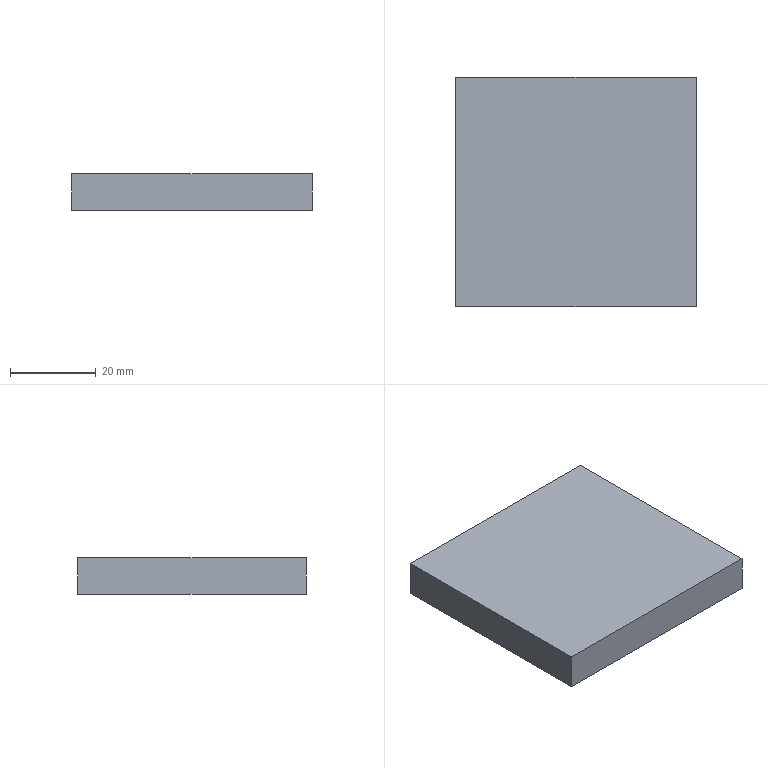NC program | NX | posted with a generic post | part box 56 x 53.3 x 8.5 mm
Lines 35 to 843 of 5023:
(刀补11_COPY_1_COPY , TOOL : D6)
N68 T12 M6
N70 G54
N72 G17 G0 G90 X5.148 Y-24.207 S9500 M3
N74 G43 Z30. H12
N76 Z1.5
N78 G94 G1 X3.722 Y-24.479 Z1.424 F1000.
N80 X1.866 Y-24.69 Z1.326
N82 X0. Y-24.76 Z1.228
N84 X-1.866 Y-24.69 Z1.13
N86 X-3.722 Y-24.479 Z1.032
N88 X-5.556 Y-24.129 Z0.935
N90 X-7.359 Y-23.641 Z0.837
N92 X-9.12 Y-23.019 Z0.739
N94 X-10.828 Y-22.267 Z0.641
N96 X-12.476 Y-21.387 Z0.543
N98 X-13.358 Y-20.839 Z0.489
N100 X-14.002 Y-20.306 Z0.445
N102 X-14.559 Y-19.684 Z0.401
N104 X-15.018 Y-18.987 Z0.357
N106 X-15.369 Y-18.228 Z0.314
N108 X-15.603 Y-17.426 Z0.27
N110 X-15.715 Y-16.598 Z0.226
N112 Y-15.974 Z0.193
N114 X-15.686 Y-15.686 Z0.178
N116 X-16.019 Y-15.72 Z0.161
N118 X-16.95 Y-15.683 Z0.112
N120 X-17.862 Y-15.492 Z0.063
N122 X-18.73 Y-15.153 Z0.014
N124 X-19.529 Y-14.675 Z-0.035
N126 X-20.239 Y-14.071 Z-0.084
N128 X-20.839 Y-13.358 Z-0.132
N130 X-21.015 Y-13.073 Z-0.15
N132 G2 X-22.44 Y-10.442 R24.75 F2000.
N134 X-24.805 Y-8.12 R3.6
N136 X-24.805 Y8.12 R26.1
N138 X-22.44 Y10.442 R3.6
N140 X-21.015 Y13.073 R24.75
N142 X-15.686 Y15.686 R5.6
N144 X-13.073 Y21.015 R5.6
N146 X13.073 Y21.015 R24.75
N148 X15.686 Y15.686 R5.6
N150 X21.015 Y13.073 R5.6
N152 X22.44 Y10.442 R24.75
N154 X24.805 Y8.12 R3.6
N156 X24.805 Y-8.12 R26.1
N158 X22.44 Y-10.442 R3.6
N160 X21.015 Y-13.073 R24.75
N162 X15.686 Y-15.686 R5.6
N164 X13.073 Y-21.015 R5.6
N166 X-13.073 Y-21.015 R24.75
N168 X-15.686 Y-15.686 R5.6
N170 X-21.015 Y-13.073 R5.6
N172 G1 X-21.106 Y-12.927 Z-0.153
N174 X-21.195 Y-12.78 Z-0.156
N176 X-21.283 Y-12.633 Z-0.159
N178 X-21.37 Y-12.485 Z-0.162
N180 X-21.457 Y-12.336 Z-0.165
N182 X-21.542 Y-12.187 Z-0.168
N184 X-21.626 Y-12.037 Z-0.171
N186 X-21.709 Y-11.886 Z-0.174
N188 X-21.791 Y-11.735 Z-0.177
N190 X-21.872 Y-11.584 Z-0.18
N192 X-21.952 Y-11.431 Z-0.183
N194 X-22.031 Y-11.279 Z-0.186
N196 X-22.109 Y-11.126 Z-0.189
N198 X-22.185 Y-10.972 Z-0.192
N200 X-22.261 Y-10.817 Z-0.195
N202 X-22.335 Y-10.663 Z-0.198
N204 X-22.437 Y-10.447 Z-0.202
N206 X-22.534 Y-10.411 Z-0.204
N208 X-22.696 Y-10.352 Z-0.207
N210 X-22.854 Y-10.286 Z-0.21
N212 X-23.009 Y-10.212 Z-0.213
N214 X-23.161 Y-10.131 Z-0.216
N216 X-23.308 Y-10.042 Z-0.219
N218 X-23.451 Y-9.947 Z-0.222
N220 X-23.589 Y-9.845 Z-0.225
N222 X-23.723 Y-9.736 Z-0.228
N224 X-23.851 Y-9.622 Z-0.231
N226 X-23.973 Y-9.501 Z-0.234
N228 X-24.089 Y-9.374 Z-0.237
N230 X-24.2 Y-9.243 Z-0.24
N232 X-24.303 Y-9.106 Z-0.243
N234 X-24.401 Y-8.964 Z-0.246
N236 X-24.491 Y-8.818 Z-0.249
N238 X-24.574 Y-8.667 Z-0.252
N240 X-24.65 Y-8.513 Z-0.255
N242 X-24.718 Y-8.356 Z-0.258
N244 X-24.779 Y-8.195 Z-0.261
N246 X-24.833 Y-8.032 Z-0.264
N248 X-24.886 Y-7.868 Z-0.267
N250 X-24.937 Y-7.704 Z-0.27
N252 X-24.987 Y-7.54 Z-0.273
N254 X-25.036 Y-7.375 Z-0.276
N256 X-25.084 Y-7.21 Z-0.279
N258 X-25.131 Y-7.044 Z-0.282
N260 X-25.177 Y-6.879 Z-0.285
N262 X-25.222 Y-6.713 Z-0.288
N264 X-25.266 Y-6.547 Z-0.291
N266 X-25.308 Y-6.38 Z-0.294
N268 X-25.35 Y-6.213 Z-0.297
N270 X-25.39 Y-6.046 Z-0.3
N272 G2 X-24.805 Y8.12 R26.1
N274 X-22.44 Y10.442 R3.6
N276 X-21.015 Y13.073 R24.75
N278 X-15.686 Y15.686 R5.6
N280 X-13.073 Y21.015 R5.6
N282 X13.073 Y21.015 R24.75
N284 X15.686 Y15.686 R5.6
N286 X21.015 Y13.073 R5.6
N288 X22.44 Y10.442 R24.75
N290 X24.805 Y8.12 R3.6
N292 X24.805 Y-8.12 R26.1
N294 X22.44 Y-10.442 R3.6
N296 X21.015 Y-13.073 R24.75
N298 X15.686 Y-15.686 R5.6
N300 X13.073 Y-21.015 R5.6
N302 X-13.073 Y-21.015 R24.75
N304 X-15.686 Y-15.686 R5.6
N306 X-21.015 Y-13.073 R5.6
N308 G1 X-21.106 Y-12.927 Z-0.303
N310 X-21.195 Y-12.78 Z-0.306
N312 X-21.283 Y-12.633 Z-0.309
N314 X-21.37 Y-12.485 Z-0.312
N316 X-21.457 Y-12.336 Z-0.315
N318 X-21.542 Y-12.187 Z-0.318
N320 X-21.626 Y-12.037 Z-0.321
N322 X-21.709 Y-11.886 Z-0.324
N324 X-21.791 Y-11.735 Z-0.327
N326 X-21.872 Y-11.584 Z-0.33
N328 X-21.952 Y-11.431 Z-0.333
N330 X-22.031 Y-11.279 Z-0.336
N332 X-22.109 Y-11.126 Z-0.339
N334 X-22.185 Y-10.972 Z-0.342
N336 X-22.261 Y-10.817 Z-0.345
N338 X-22.335 Y-10.663 Z-0.348
N340 X-22.437 Y-10.447 Z-0.352
N342 X-22.534 Y-10.411 Z-0.354
N344 X-22.696 Y-10.352 Z-0.357
N346 X-22.854 Y-10.286 Z-0.36
N348 X-23.009 Y-10.212 Z-0.363
N350 X-23.161 Y-10.131 Z-0.366
N352 X-23.308 Y-10.042 Z-0.369
N354 X-23.451 Y-9.947 Z-0.372
N356 X-23.589 Y-9.845 Z-0.375
N358 X-23.723 Y-9.736 Z-0.378
N360 X-23.851 Y-9.622 Z-0.381
N362 X-23.973 Y-9.501 Z-0.384
N364 X-24.089 Y-9.374 Z-0.387
N366 X-24.2 Y-9.243 Z-0.39
N368 X-24.303 Y-9.106 Z-0.393
N370 X-24.401 Y-8.964 Z-0.396
N372 X-24.491 Y-8.818 Z-0.399
N374 X-24.574 Y-8.667 Z-0.402
N376 X-24.65 Y-8.513 Z-0.405
N378 X-24.718 Y-8.356 Z-0.408
N380 X-24.779 Y-8.195 Z-0.411
N382 X-24.833 Y-8.032 Z-0.414
N384 X-24.886 Y-7.868 Z-0.417
N386 X-24.937 Y-7.704 Z-0.42
N388 X-24.987 Y-7.54 Z-0.423
N390 X-25.036 Y-7.375 Z-0.426
N392 X-25.084 Y-7.21 Z-0.429
N394 X-25.131 Y-7.044 Z-0.432
N396 X-25.177 Y-6.879 Z-0.435
N398 X-25.222 Y-6.713 Z-0.438
N400 X-25.266 Y-6.547 Z-0.441
N402 X-25.308 Y-6.38 Z-0.444
N404 X-25.35 Y-6.213 Z-0.447
N406 X-25.39 Y-6.046 Z-0.45
N408 G2 X-24.805 Y8.12 R26.1
N410 X-22.44 Y10.442 R3.6
N412 X-21.015 Y13.073 R24.75
N414 X-15.686 Y15.686 R5.6
N416 X-13.073 Y21.015 R5.6
N418 X13.073 Y21.015 R24.75
N420 X15.686 Y15.686 R5.6
N422 X21.015 Y13.073 R5.6
N424 X22.44 Y10.442 R24.75
N426 X24.805 Y8.12 R3.6
N428 X24.805 Y-8.12 R26.1
N430 X22.44 Y-10.442 R3.6
N432 X21.015 Y-13.073 R24.75
N434 X15.686 Y-15.686 R5.6
N436 X13.073 Y-21.015 R5.6
N438 X-13.073 Y-21.015 R24.75
N440 X-15.686 Y-15.686 R5.6
N442 X-21.015 Y-13.073 R5.6
N444 G1 X-21.106 Y-12.927 Z-0.453
N446 X-21.195 Y-12.78 Z-0.456
N448 X-21.283 Y-12.633 Z-0.459
N450 X-21.37 Y-12.485 Z-0.462
N452 X-21.457 Y-12.336 Z-0.465
N454 X-21.542 Y-12.187 Z-0.468
N456 X-21.626 Y-12.037 Z-0.471
N458 X-21.709 Y-11.886 Z-0.474
N460 X-21.791 Y-11.735 Z-0.477
N462 X-21.872 Y-11.584 Z-0.48
N464 X-21.952 Y-11.431 Z-0.483
N466 X-22.031 Y-11.279 Z-0.486
N468 X-22.109 Y-11.126 Z-0.489
N470 X-22.185 Y-10.972 Z-0.492
N472 X-22.261 Y-10.817 Z-0.495
N474 X-22.335 Y-10.663 Z-0.498
N476 X-22.437 Y-10.447 Z-0.502
N478 X-22.534 Y-10.411 Z-0.504
N480 X-22.696 Y-10.352 Z-0.507
N482 X-22.854 Y-10.286 Z-0.51
N484 X-23.009 Y-10.212 Z-0.513
N486 X-23.161 Y-10.131 Z-0.516
N488 X-23.308 Y-10.042 Z-0.519
N490 X-23.451 Y-9.947 Z-0.522
N492 X-23.589 Y-9.845 Z-0.525
N494 X-23.723 Y-9.736 Z-0.528
N496 X-23.851 Y-9.622 Z-0.531
N498 X-23.973 Y-9.501 Z-0.534
N500 X-24.089 Y-9.374 Z-0.537
N502 X-24.2 Y-9.243 Z-0.54
N504 X-24.303 Y-9.106 Z-0.543
N506 X-24.401 Y-8.964 Z-0.546
N508 X-24.491 Y-8.818 Z-0.549
N510 X-24.574 Y-8.667 Z-0.552
N512 X-24.65 Y-8.513 Z-0.555
N514 X-24.718 Y-8.356 Z-0.558
N516 X-24.779 Y-8.195 Z-0.561
N518 X-24.833 Y-8.032 Z-0.564
N520 X-24.886 Y-7.868 Z-0.567
N522 X-24.937 Y-7.704 Z-0.57
N524 X-24.987 Y-7.54 Z-0.573
N526 X-25.036 Y-7.375 Z-0.576
N528 X-25.084 Y-7.21 Z-0.579
N530 X-25.131 Y-7.044 Z-0.582
N532 X-25.177 Y-6.879 Z-0.585
N534 X-25.222 Y-6.713 Z-0.588
N536 X-25.266 Y-6.547 Z-0.591
N538 X-25.308 Y-6.38 Z-0.594
N540 X-25.35 Y-6.213 Z-0.597
N542 X-25.39 Y-6.046 Z-0.6
N544 G2 X-24.805 Y8.12 R26.1
N546 X-22.44 Y10.442 R3.6
N548 X-21.015 Y13.073 R24.75
N550 X-15.686 Y15.686 R5.6
N552 X-13.073 Y21.015 R5.6
N554 X13.073 Y21.015 R24.75
N556 X15.686 Y15.686 R5.6
N558 X21.015 Y13.073 R5.6
N560 X22.44 Y10.442 R24.75
N562 X24.805 Y8.12 R3.6
N564 X24.805 Y-8.12 R26.1
N566 X22.44 Y-10.442 R3.6
N568 X21.015 Y-13.073 R24.75
N570 X15.686 Y-15.686 R5.6
N572 X13.073 Y-21.015 R5.6
N574 X-13.073 Y-21.015 R24.75
N576 X-15.686 Y-15.686 R5.6
N578 X-21.015 Y-13.073 R5.6
N580 G1 X-21.106 Y-12.927 Z-0.603
N582 X-21.195 Y-12.78 Z-0.606
N584 X-21.283 Y-12.633 Z-0.609
N586 X-21.37 Y-12.485 Z-0.612
N588 X-21.457 Y-12.336 Z-0.615
N590 X-21.542 Y-12.187 Z-0.618
N592 X-21.626 Y-12.037 Z-0.621
N594 X-21.709 Y-11.886 Z-0.624
N596 X-21.791 Y-11.735 Z-0.627
N598 X-21.872 Y-11.584 Z-0.63
N600 X-21.952 Y-11.431 Z-0.633
N602 X-22.031 Y-11.279 Z-0.636
N604 X-22.109 Y-11.126 Z-0.639
N606 X-22.185 Y-10.972 Z-0.642
N608 X-22.261 Y-10.817 Z-0.645
N610 X-22.335 Y-10.663 Z-0.648
N612 X-22.437 Y-10.447 Z-0.652
N614 X-22.534 Y-10.411 Z-0.654
N616 X-22.696 Y-10.352 Z-0.657
N618 X-22.854 Y-10.286 Z-0.66
N620 X-23.009 Y-10.212 Z-0.663
N622 X-23.161 Y-10.131 Z-0.666
N624 X-23.308 Y-10.042 Z-0.669
N626 X-23.451 Y-9.947 Z-0.672
N628 X-23.589 Y-9.845 Z-0.675
N630 X-23.723 Y-9.736 Z-0.678
N632 X-23.851 Y-9.622 Z-0.681
N634 X-23.973 Y-9.501 Z-0.684
N636 X-24.089 Y-9.374 Z-0.687
N638 X-24.2 Y-9.243 Z-0.69
N640 X-24.303 Y-9.106 Z-0.693
N642 X-24.401 Y-8.964 Z-0.696
N644 X-24.491 Y-8.818 Z-0.699
N646 X-24.574 Y-8.667 Z-0.702
N648 X-24.65 Y-8.513 Z-0.705
N650 X-24.718 Y-8.356 Z-0.708
N652 X-24.779 Y-8.195 Z-0.711
N654 X-24.833 Y-8.032 Z-0.714
N656 X-24.886 Y-7.868 Z-0.717
N658 X-24.937 Y-7.704 Z-0.72
N660 X-24.987 Y-7.54 Z-0.723
N662 X-25.036 Y-7.375 Z-0.726
N664 X-25.084 Y-7.21 Z-0.729
N666 X-25.131 Y-7.044 Z-0.732
N668 X-25.177 Y-6.879 Z-0.735
N670 X-25.222 Y-6.713 Z-0.738
N672 X-25.266 Y-6.547 Z-0.741
N674 X-25.308 Y-6.38 Z-0.744
N676 X-25.35 Y-6.213 Z-0.747
N678 X-25.39 Y-6.046 Z-0.75
N680 G2 X-24.805 Y8.12 R26.1
N682 X-22.44 Y10.442 R3.6
N684 X-21.015 Y13.073 R24.75
N686 X-15.686 Y15.686 R5.6
N688 X-13.073 Y21.015 R5.6
N690 X13.073 Y21.015 R24.75
N692 X15.686 Y15.686 R5.6
N694 X21.015 Y13.073 R5.6
N696 X22.44 Y10.442 R24.75
N698 X24.805 Y8.12 R3.6
N700 X24.805 Y-8.12 R26.1
N702 X22.44 Y-10.442 R3.6
N704 X21.015 Y-13.073 R24.75
N706 X15.686 Y-15.686 R5.6
N708 X13.073 Y-21.015 R5.6
N710 X-13.073 Y-21.015 R24.75
N712 X-15.686 Y-15.686 R5.6
N714 X-21.015 Y-13.073 R5.6
N716 G1 X-21.106 Y-12.927 Z-0.753
N718 X-21.195 Y-12.78 Z-0.756
N720 X-21.283 Y-12.633 Z-0.759
N722 X-21.37 Y-12.485 Z-0.762
N724 X-21.457 Y-12.336 Z-0.765
N726 X-21.542 Y-12.187 Z-0.768
N728 X-21.626 Y-12.037 Z-0.771
N730 X-21.709 Y-11.886 Z-0.774
N732 X-21.791 Y-11.735 Z-0.777
N734 X-21.872 Y-11.584 Z-0.78
N736 X-21.952 Y-11.431 Z-0.783
N738 X-22.031 Y-11.279 Z-0.786
N740 X-22.109 Y-11.126 Z-0.789
N742 X-22.185 Y-10.972 Z-0.792
N744 X-22.261 Y-10.817 Z-0.795
N746 X-22.335 Y-10.663 Z-0.798
N748 X-22.437 Y-10.447 Z-0.802
N750 X-22.534 Y-10.411 Z-0.804
N752 X-22.696 Y-10.352 Z-0.807
N754 X-22.854 Y-10.286 Z-0.81
N756 X-23.009 Y-10.212 Z-0.813
N758 X-23.161 Y-10.131 Z-0.816
N760 X-23.308 Y-10.042 Z-0.819
N762 X-23.451 Y-9.947 Z-0.822
N764 X-23.589 Y-9.845 Z-0.825
N766 X-23.723 Y-9.736 Z-0.828
N768 X-23.851 Y-9.622 Z-0.831
N770 X-23.973 Y-9.501 Z-0.834
N772 X-24.089 Y-9.374 Z-0.837
N774 X-24.2 Y-9.243 Z-0.84
N776 X-24.303 Y-9.106 Z-0.843
N778 X-24.401 Y-8.964 Z-0.846
N780 X-24.491 Y-8.818 Z-0.849
N782 X-24.574 Y-8.667 Z-0.852
N784 X-24.65 Y-8.513 Z-0.855
N786 X-24.718 Y-8.356 Z-0.858
N788 X-24.779 Y-8.195 Z-0.861
N790 X-24.833 Y-8.032 Z-0.864
N792 X-24.886 Y-7.868 Z-0.867
N794 X-24.937 Y-7.704 Z-0.87
N796 X-24.987 Y-7.54 Z-0.873
N798 X-25.036 Y-7.375 Z-0.876
N800 X-25.084 Y-7.21 Z-0.879
N802 X-25.131 Y-7.044 Z-0.882
N804 X-25.177 Y-6.879 Z-0.885
N806 X-25.222 Y-6.713 Z-0.888
N808 X-25.266 Y-6.547 Z-0.891
N810 X-25.308 Y-6.38 Z-0.894
N812 X-25.35 Y-6.213 Z-0.897
N814 X-25.39 Y-6.046 Z-0.9
N816 G2 X-24.805 Y8.12 R26.1
N818 X-22.44 Y10.442 R3.6
N820 X-21.015 Y13.073 R24.75
N822 X-15.686 Y15.686 R5.6
N824 X-13.073 Y21.015 R5.6
N826 X13.073 Y21.015 R24.75
N828 X15.686 Y15.686 R5.6
N830 X21.015 Y13.073 R5.6
N832 X22.44 Y10.442 R24.75
N834 X24.805 Y8.12 R3.6
N836 X24.805 Y-8.12 R26.1
N838 X22.44 Y-10.442 R3.6
N840 X21.015 Y-13.073 R24.75
N842 X15.686 Y-15.686 R5.6
N844 X13.073 Y-21.015 R5.6
N846 X-13.073 Y-21.015 R24.75
N848 X-15.686 Y-15.686 R5.6
N850 X-21.015 Y-13.073 R5.6
N852 G1 X-21.106 Y-12.927 Z-0.903
N854 X-21.195 Y-12.78 Z-0.906
N856 X-21.283 Y-12.633 Z-0.909
N858 X-21.37 Y-12.485 Z-0.912
N860 X-21.457 Y-12.336 Z-0.915
N862 X-21.542 Y-12.187 Z-0.918
N864 X-21.626 Y-12.037 Z-0.921
N866 X-21.709 Y-11.886 Z-0.924
N868 X-21.791 Y-11.735 Z-0.927
N870 X-21.872 Y-11.584 Z-0.93
N872 X-21.952 Y-11.431 Z-0.933
N874 X-22.031 Y-11.279 Z-0.936
N876 X-22.109 Y-11.126 Z-0.939
N878 X-22.185 Y-10.972 Z-0.942
N880 X-22.261 Y-10.817 Z-0.945
N882 X-22.335 Y-10.663 Z-0.948
N884 X-22.437 Y-10.447 Z-0.952
N886 X-22.534 Y-10.411 Z-0.954
N888 X-22.696 Y-10.352 Z-0.957
N890 X-22.854 Y-10.286 Z-0.96
N892 X-23.009 Y-10.212 Z-0.963
N894 X-23.161 Y-10.131 Z-0.966
N896 X-23.308 Y-10.042 Z-0.969
N898 X-23.451 Y-9.947 Z-0.972
N900 X-23.589 Y-9.845 Z-0.975
N902 X-23.723 Y-9.736 Z-0.978
N904 X-23.851 Y-9.622 Z-0.981
N906 X-23.973 Y-9.501 Z-0.984
N908 X-24.089 Y-9.374 Z-0.987
N910 X-24.2 Y-9.243 Z-0.99
N912 X-24.303 Y-9.106 Z-0.993
N914 X-24.401 Y-8.964 Z-0.996
N916 X-24.491 Y-8.818 Z-0.999
N918 X-24.574 Y-8.667 Z-1.002
N920 X-24.65 Y-8.513 Z-1.005
N922 X-24.718 Y-8.356 Z-1.008
N924 X-24.779 Y-8.195 Z-1.011
N926 X-24.833 Y-8.032 Z-1.014
N928 X-24.886 Y-7.868 Z-1.017
N930 X-24.937 Y-7.704 Z-1.02
N932 X-24.987 Y-7.54 Z-1.023
N934 X-25.036 Y-7.375 Z-1.026
N936 X-25.084 Y-7.21 Z-1.029
N938 X-25.131 Y-7.044 Z-1.032
N940 X-25.177 Y-6.879 Z-1.035
N942 X-25.222 Y-6.713 Z-1.038
N944 X-25.266 Y-6.547 Z-1.041
N946 X-25.308 Y-6.38 Z-1.044
N948 X-25.35 Y-6.213 Z-1.047
N950 X-25.39 Y-6.046 Z-1.05
N952 G2 X-24.805 Y8.12 R26.1
N954 X-22.44 Y10.442 R3.6
N956 X-21.015 Y13.073 R24.75
N958 X-15.686 Y15.686 R5.6
N960 X-13.073 Y21.015 R5.6
N962 X13.073 Y21.015 R24.75
N964 X15.686 Y15.686 R5.6
N966 X21.015 Y13.073 R5.6
N968 X22.44 Y10.442 R24.75
N970 X24.805 Y8.12 R3.6
N972 X24.805 Y-8.12 R26.1
N974 X22.44 Y-10.442 R3.6
N976 X21.015 Y-13.073 R24.75
N978 X15.686 Y-15.686 R5.6
N980 X13.073 Y-21.015 R5.6
N982 X-13.073 Y-21.015 R24.75
N984 X-15.686 Y-15.686 R5.6
N986 X-21.015 Y-13.073 R5.6
N988 G1 X-21.106 Y-12.927 Z-1.053
N990 X-21.195 Y-12.78 Z-1.056
N992 X-21.283 Y-12.633 Z-1.059
N994 X-21.37 Y-12.485 Z-1.062
N996 X-21.457 Y-12.336 Z-1.065
N998 X-21.542 Y-12.187 Z-1.068
N1000 X-21.626 Y-12.037 Z-1.071
N1002 X-21.709 Y-11.886 Z-1.074
N1004 X-21.791 Y-11.735 Z-1.077
N1006 X-21.872 Y-11.584 Z-1.08
N1008 X-21.952 Y-11.431 Z-1.083
N1010 X-22.031 Y-11.279 Z-1.086
N1012 X-22.109 Y-11.126 Z-1.089
N1014 X-22.185 Y-10.972 Z-1.092
N1016 X-22.261 Y-10.817 Z-1.095
N1018 X-22.335 Y-10.663 Z-1.098
N1020 X-22.437 Y-10.447 Z-1.102
N1022 X-22.534 Y-10.411 Z-1.104
N1024 X-22.696 Y-10.352 Z-1.107
N1026 X-22.854 Y-10.286 Z-1.11
N1028 X-23.009 Y-10.212 Z-1.113
N1030 X-23.161 Y-10.131 Z-1.116
N1032 X-23.308 Y-10.042 Z-1.119
N1034 X-23.451 Y-9.947 Z-1.122
N1036 X-23.589 Y-9.845 Z-1.125
N1038 X-23.723 Y-9.736 Z-1.128
N1040 X-23.851 Y-9.622 Z-1.131
N1042 X-23.973 Y-9.501 Z-1.134
N1044 X-24.089 Y-9.374 Z-1.137
N1046 X-24.2 Y-9.243 Z-1.14
N1048 X-24.303 Y-9.106 Z-1.143
N1050 X-24.401 Y-8.964 Z-1.146
N1052 X-24.491 Y-8.818 Z-1.149
N1054 X-24.574 Y-8.667 Z-1.152
N1056 X-24.65 Y-8.513 Z-1.155
N1058 X-24.718 Y-8.356 Z-1.158
N1060 X-24.779 Y-8.195 Z-1.161
N1062 X-24.833 Y-8.032 Z-1.164
N1064 X-24.886 Y-7.868 Z-1.167
N1066 X-24.937 Y-7.704 Z-1.17
N1068 X-24.987 Y-7.54 Z-1.173
N1070 X-25.036 Y-7.375 Z-1.176
N1072 X-25.084 Y-7.21 Z-1.179
N1074 X-25.131 Y-7.044 Z-1.182
N1076 X-25.177 Y-6.879 Z-1.185
N1078 X-25.222 Y-6.713 Z-1.188
N1080 X-25.266 Y-6.547 Z-1.191
N1082 X-25.308 Y-6.38 Z-1.194
N1084 X-25.35 Y-6.213 Z-1.197
N1086 X-25.39 Y-6.046 Z-1.2
N1088 G2 X-24.805 Y8.12 R26.1
N1090 X-22.44 Y10.442 R3.6
N1092 X-21.015 Y13.073 R24.75
N1094 X-15.686 Y15.686 R5.6
N1096 X-13.073 Y21.015 R5.6
N1098 X13.073 Y21.015 R24.75
N1100 X15.686 Y15.686 R5.6
N1102 X21.015 Y13.073 R5.6
N1104 X22.44 Y10.442 R24.75
N1106 X24.805 Y8.12 R3.6
N1108 X24.805 Y-8.12 R26.1
N1110 X22.44 Y-10.442 R3.6
N1112 X21.015 Y-13.073 R24.75
N1114 X15.686 Y-15.686 R5.6
N1116 X13.073 Y-21.015 R5.6
N1118 X-13.073 Y-21.015 R24.75
N1120 X-15.686 Y-15.686 R5.6
N1122 X-21.015 Y-13.073 R5.6
N1124 G1 X-21.106 Y-12.927 Z-1.203
N1126 X-21.195 Y-12.78 Z-1.206
N1128 X-21.283 Y-12.633 Z-1.209
N1130 X-21.37 Y-12.485 Z-1.212
N1132 X-21.457 Y-12.336 Z-1.215
N1134 X-21.542 Y-12.187 Z-1.218
N1136 X-21.626 Y-12.037 Z-1.221
N1138 X-21.709 Y-11.886 Z-1.224
N1140 X-21.791 Y-11.735 Z-1.227
N1142 X-21.872 Y-11.584 Z-1.23
N1144 X-21.952 Y-11.431 Z-1.233
N1146 X-22.031 Y-11.279 Z-1.236
N1148 X-22.109 Y-11.126 Z-1.239
N1150 X-22.185 Y-10.972 Z-1.242
N1152 X-22.261 Y-10.817 Z-1.245
N1154 X-22.335 Y-10.663 Z-1.248
N1156 X-22.437 Y-10.447 Z-1.252
N1158 X-22.534 Y-10.411 Z-1.254
N1160 X-22.696 Y-10.352 Z-1.257
N1162 X-22.854 Y-10.286 Z-1.26
N1164 X-23.009 Y-10.212 Z-1.263
N1166 X-23.161 Y-10.131 Z-1.266
N1168 X-23.308 Y-10.042 Z-1.269
N1170 X-23.451 Y-9.947 Z-1.272
N1172 X-23.589 Y-9.845 Z-1.275
N1174 X-23.723 Y-9.736 Z-1.278
N1176 X-23.851 Y-9.622 Z-1.281
N1178 X-23.973 Y-9.501 Z-1.284
N1180 X-24.089 Y-9.374 Z-1.287
N1182 X-24.2 Y-9.243 Z-1.29
N1184 X-24.303 Y-9.106 Z-1.293
N1186 X-24.401 Y-8.964 Z-1.296
N1188 X-24.491 Y-8.818 Z-1.299
N1190 X-24.574 Y-8.667 Z-1.302
N1192 X-24.65 Y-8.513 Z-1.305
N1194 X-24.718 Y-8.356 Z-1.308
N1196 X-24.779 Y-8.195 Z-1.311
N1198 X-24.833 Y-8.032 Z-1.314
N1200 X-24.886 Y-7.868 Z-1.317
N1202 X-24.937 Y-7.704 Z-1.32
N1204 X-24.987 Y-7.54 Z-1.323
N1206 X-25.036 Y-7.375 Z-1.326
N1208 X-25.084 Y-7.21 Z-1.329
N1210 X-25.131 Y-7.044 Z-1.332
N1212 X-25.177 Y-6.879 Z-1.335
N1214 X-25.222 Y-6.713 Z-1.338
N1216 X-25.266 Y-6.547 Z-1.341
N1218 X-25.308 Y-6.38 Z-1.344
N1220 X-25.35 Y-6.213 Z-1.347
N1222 X-25.39 Y-6.046 Z-1.35
N1224 G2 X-24.805 Y8.12 R26.1
N1226 X-22.44 Y10.442 R3.6
N1228 X-21.015 Y13.073 R24.75
N1230 X-15.686 Y15.686 R5.6
N1232 X-13.073 Y21.015 R5.6
N1234 X13.073 Y21.015 R24.75
N1236 X15.686 Y15.686 R5.6
N1238 X21.015 Y13.073 R5.6
N1240 X22.44 Y10.442 R24.75
N1242 X24.805 Y8.12 R3.6
N1244 X24.805 Y-8.12 R26.1
N1246 X22.44 Y-10.442 R3.6
N1248 X21.015 Y-13.073 R24.75
N1250 X15.686 Y-15.686 R5.6
N1252 X13.073 Y-21.015 R5.6
N1254 X-13.073 Y-21.015 R24.75
N1256 X-15.686 Y-15.686 R5.6
N1258 X-21.015 Y-13.073 R5.6
N1260 G1 X-21.106 Y-12.927 Z-1.353
N1262 X-21.195 Y-12.78 Z-1.356
N1264 X-21.283 Y-12.633 Z-1.359
N1266 X-21.37 Y-12.485 Z-1.362
N1268 X-21.457 Y-12.336 Z-1.365
N1270 X-21.542 Y-12.187 Z-1.368
N1272 X-21.626 Y-12.037 Z-1.371
N1274 X-21.709 Y-11.886 Z-1.374
N1276 X-21.791 Y-11.735 Z-1.377
N1278 X-21.872 Y-11.584 Z-1.38
N1280 X-21.952 Y-11.431 Z-1.383
N1282 X-22.031 Y-11.279 Z-1.386
N1284 X-22.109 Y-11.126 Z-1.389
N1286 X-22.185 Y-10.972 Z-1.392
N1288 X-22.261 Y-10.817 Z-1.395
N1290 X-22.335 Y-10.663 Z-1.398
N1292 X-22.437 Y-10.447 Z-1.402
N1294 X-22.534 Y-10.411 Z-1.404
N1296 X-22.696 Y-10.352 Z-1.407
N1298 X-22.854 Y-10.286 Z-1.41
N1300 X-23.009 Y-10.212 Z-1.413
N1302 X-23.161 Y-10.131 Z-1.416
N1304 X-23.308 Y-10.042 Z-1.419
N1306 X-23.451 Y-9.947 Z-1.422
N1308 X-23.589 Y-9.845 Z-1.425
N1310 X-23.723 Y-9.736 Z-1.428
N1312 X-23.851 Y-9.622 Z-1.431
N1314 X-23.973 Y-9.501 Z-1.434
N1316 X-24.089 Y-9.374 Z-1.437
N1318 X-24.2 Y-9.243 Z-1.44
N1320 X-24.303 Y-9.106 Z-1.443
N1322 X-24.401 Y-8.964 Z-1.446
N1324 X-24.491 Y-8.818 Z-1.449
N1326 X-24.574 Y-8.667 Z-1.452
N1328 X-24.65 Y-8.513 Z-1.455
N1330 X-24.718 Y-8.356 Z-1.458
N1332 X-24.779 Y-8.195 Z-1.461
N1334 X-24.833 Y-8.032 Z-1.464
N1336 X-24.886 Y-7.868 Z-1.467
N1338 X-24.937 Y-7.704 Z-1.47
N1340 X-24.987 Y-7.54 Z-1.473
N1342 X-25.036 Y-7.375 Z-1.476
N1344 X-25.084 Y-7.21 Z-1.479
N1346 X-25.131 Y-7.044 Z-1.482
N1348 X-25.177 Y-6.879 Z-1.485
N1350 X-25.222 Y-6.713 Z-1.488
N1352 X-25.266 Y-6.547 Z-1.491
N1354 X-25.308 Y-6.38 Z-1.494
N1356 X-25.35 Y-6.213 Z-1.497
N1358 X-25.39 Y-6.046 Z-1.5
N1360 G2 X-24.805 Y8.12 R26.1
N1362 X-22.44 Y10.442 R3.6
N1364 X-21.015 Y13.073 R24.75
N1366 X-15.686 Y15.686 R5.6
N1368 X-13.073 Y21.015 R5.6
N1370 X13.073 Y21.015 R24.75
N1372 X15.686 Y15.686 R5.6
N1374 X21.015 Y13.073 R5.6
N1376 X22.44 Y10.442 R24.75
N1378 X24.805 Y8.12 R3.6
N1380 X24.805 Y-8.12 R26.1
N1382 X22.44 Y-10.442 R3.6
N1384 X21.015 Y-13.073 R24.75
N1386 X15.686 Y-15.686 R5.6
N1388 X13.073 Y-21.015 R5.6
N1390 X-13.073 Y-21.015 R24.75
N1392 X-15.686 Y-15.686 R5.6
N1394 X-21.015 Y-13.073 R5.6
N1396 G1 X-21.106 Y-12.927 Z-1.503
N1398 X-21.195 Y-12.78 Z-1.506
N1400 X-21.283 Y-12.633 Z-1.509
N1402 X-21.37 Y-12.485 Z-1.512
N1404 X-21.457 Y-12.336 Z-1.515
N1406 X-21.542 Y-12.187 Z-1.518
N1408 X-21.626 Y-12.037 Z-1.521
N1410 X-21.709 Y-11.886 Z-1.524
N1412 X-21.791 Y-11.735 Z-1.527
N1414 X-21.872 Y-11.584 Z-1.53
N1416 X-21.952 Y-11.431 Z-1.533
N1418 X-22.031 Y-11.279 Z-1.536
N1420 X-22.109 Y-11.126 Z-1.539
N1422 X-22.185 Y-10.972 Z-1.542
N1424 X-22.261 Y-10.817 Z-1.545
N1426 X-22.335 Y-10.663 Z-1.548
N1428 X-22.437 Y-10.447 Z-1.552
N1430 X-22.534 Y-10.411 Z-1.554
N1432 X-22.696 Y-10.352 Z-1.557
N1434 X-22.854 Y-10.286 Z-1.56
N1436 X-23.009 Y-10.212 Z-1.563
N1438 X-23.161 Y-10.131 Z-1.566
N1440 X-23.308 Y-10.042 Z-1.569
N1442 X-23.451 Y-9.947 Z-1.572
N1444 X-23.589 Y-9.845 Z-1.575
N1446 X-23.723 Y-9.736 Z-1.578
N1448 X-23.851 Y-9.622 Z-1.581
N1450 X-23.973 Y-9.501 Z-1.584
N1452 X-24.089 Y-9.374 Z-1.587
N1454 X-24.2 Y-9.243 Z-1.59
N1456 X-24.303 Y-9.106 Z-1.593
N1458 X-24.401 Y-8.964 Z-1.596
N1460 X-24.491 Y-8.818 Z-1.599
N1462 X-24.574 Y-8.667 Z-1.602
N1464 X-24.65 Y-8.513 Z-1.605
N1466 X-24.718 Y-8.356 Z-1.608
N1468 X-24.779 Y-8.195 Z-1.611
N1470 X-24.833 Y-8.032 Z-1.614
N1472 X-24.886 Y-7.868 Z-1.617
N1474 X-24.937 Y-7.704 Z-1.62
N1476 X-24.987 Y-7.54 Z-1.623
N1478 X-25.036 Y-7.375 Z-1.626
N1480 X-25.084 Y-7.21 Z-1.629
N1482 X-25.131 Y-7.044 Z-1.632
N1484 X-25.177 Y-6.879 Z-1.635
N1486 X-25.222 Y-6.713 Z-1.638
N1488 X-25.266 Y-6.547 Z-1.641
N1490 X-25.308 Y-6.38 Z-1.644
N1492 X-25.35 Y-6.213 Z-1.647
N1494 X-25.39 Y-6.046 Z-1.65
N1496 G2 X-24.805 Y8.12 R26.1
N1498 X-22.44 Y10.442 R3.6
N1500 X-21.015 Y13.073 R24.75
N1502 X-15.686 Y15.686 R5.6
N1504 X-13.073 Y21.015 R5.6
N1506 X13.073 Y21.015 R24.75
N1508 X15.686 Y15.686 R5.6
N1510 X21.015 Y13.073 R5.6
N1512 X22.44 Y10.442 R24.75
N1514 X24.805 Y8.12 R3.6
N1516 X24.805 Y-8.12 R26.1
N1518 X22.44 Y-10.442 R3.6
N1520 X21.015 Y-13.073 R24.75
N1522 X15.686 Y-15.686 R5.6
N1524 X13.073 Y-21.015 R5.6
N1526 X-13.073 Y-21.015 R24.75
N1528 X-15.686 Y-15.686 R5.6
N1530 X-21.015 Y-13.073 R5.6
N1532 G1 X-21.106 Y-12.927 Z-1.653
N1534 X-21.195 Y-12.78 Z-1.656
N1536 X-21.283 Y-12.633 Z-1.659
N1538 X-21.37 Y-12.485 Z-1.662
N1540 X-21.457 Y-12.336 Z-1.665
N1542 X-21.542 Y-12.187 Z-1.668
N1544 X-21.626 Y-12.037 Z-1.671
N1546 X-21.709 Y-11.886 Z-1.674
N1548 X-21.791 Y-11.735 Z-1.677
N1550 X-21.872 Y-11.584 Z-1.68
N1552 X-21.952 Y-11.431 Z-1.683
N1554 X-22.031 Y-11.279 Z-1.686
N1556 X-22.109 Y-11.126 Z-1.689
N1558 X-22.185 Y-10.972 Z-1.692
N1560 X-22.261 Y-10.817 Z-1.695
N1562 X-22.335 Y-10.663 Z-1.698
N1564 X-22.437 Y-10.447 Z-1.702
N1566 X-22.534 Y-10.411 Z-1.704
N1568 X-22.696 Y-10.352 Z-1.707
N1570 X-22.854 Y-10.286 Z-1.71
N1572 X-23.009 Y-10.212 Z-1.713
N1574 X-23.161 Y-10.131 Z-1.716
N1576 X-23.308 Y-10.042 Z-1.719
N1578 X-23.451 Y-9.947 Z-1.722
N1580 X-23.589 Y-9.845 Z-1.725
N1582 X-23.723 Y-9.736 Z-1.728
N1584 X-23.851 Y-9.622 Z-1.731
N1586 X-23.973 Y-9.501 Z-1.734
N1588 X-24.089 Y-9.374 Z-1.737
N1590 X-24.2 Y-9.243 Z-1.74
N1592 X-24.303 Y-9.106 Z-1.743
N1594 X-24.401 Y-8.964 Z-1.746
N1596 X-24.491 Y-8.818 Z-1.749
N1598 X-24.574 Y-8.667 Z-1.752
N1600 X-24.65 Y-8.513 Z-1.755
N1602 X-24.718 Y-8.356 Z-1.758
N1604 X-24.779 Y-8.195 Z-1.761
N1606 X-24.833 Y-8.032 Z-1.764
N1608 X-24.886 Y-7.868 Z-1.767
N1610 X-24.937 Y-7.704 Z-1.77
N1612 X-24.987 Y-7.54 Z-1.773
N1614 X-25.036 Y-7.375 Z-1.776
N1616 X-25.084 Y-7.21 Z-1.779
N1618 X-25.131 Y-7.044 Z-1.782
N1620 X-25.177 Y-6.879 Z-1.785
N1622 X-25.222 Y-6.713 Z-1.788
N1624 X-25.266 Y-6.547 Z-1.791
N1626 X-25.308 Y-6.38 Z-1.794
N1628 X-25.35 Y-6.213 Z-1.797
N1630 X-25.39 Y-6.046 Z-1.8
N1632 G2 X-24.805 Y8.12 R26.1
N1634 X-22.44 Y10.442 R3.6
N1636 X-21.015 Y13.073 R24.75
N1638 X-15.686 Y15.686 R5.6
N1640 X-13.073 Y21.015 R5.6
N1642 X13.073 Y21.015 R24.75
N1644 X15.686 Y15.686 R5.6
N1646 X21.015 Y13.073 R5.6
N1648 X22.44 Y10.442 R24.75
N1650 X24.805 Y8.12 R3.6
N1652 X24.805 Y-8.12 R26.1
N1654 X22.44 Y-10.442 R3.6
N1656 X21.015 Y-13.073 R24.75
N1658 X15.686 Y-15.686 R5.6
N1660 X13.073 Y-21.015 R5.6
N1662 X-13.073 Y-21.015 R24.75
N1664 X-15.686 Y-15.686 R5.6
N1666 X-21.015 Y-13.073 R5.6
N1668 G1 X-21.106 Y-12.927 Z-1.803
N1670 X-21.195 Y-12.78 Z-1.806
N1672 X-21.283 Y-12.633 Z-1.809
N1674 X-21.37 Y-12.485 Z-1.812
N1676 X-21.457 Y-12.336 Z-1.815
N1678 X-21.542 Y-12.187 Z-1.818